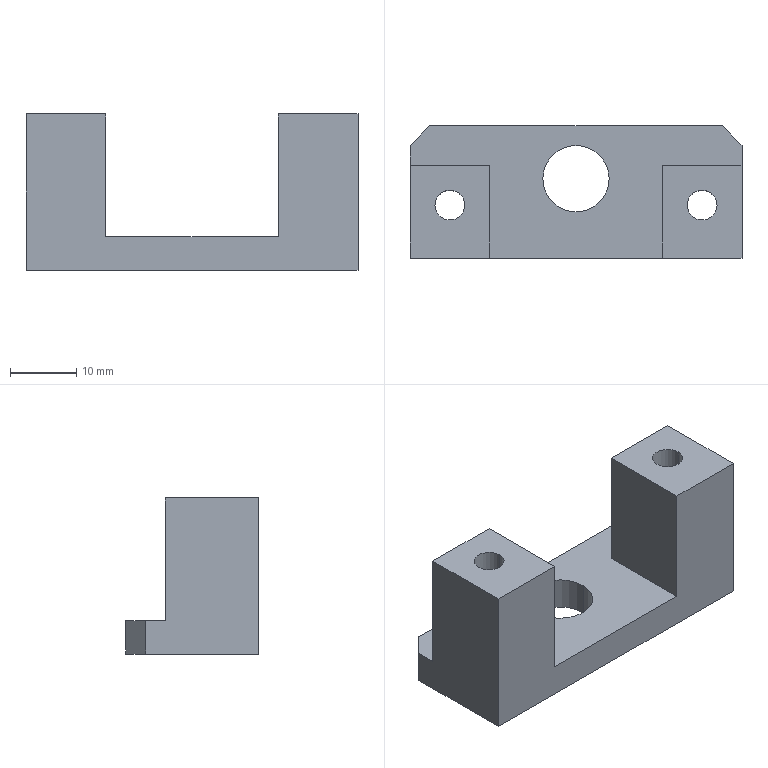Part | STEP file | slider cylinder plate | 1 solid | 26 faces | box 50 x 20 x 23.5 mm | volume 9756 mm3 | plane 16 | cylinder 10 | commonest cylinder face diameters 4.5 x4 8 x4 10 x2